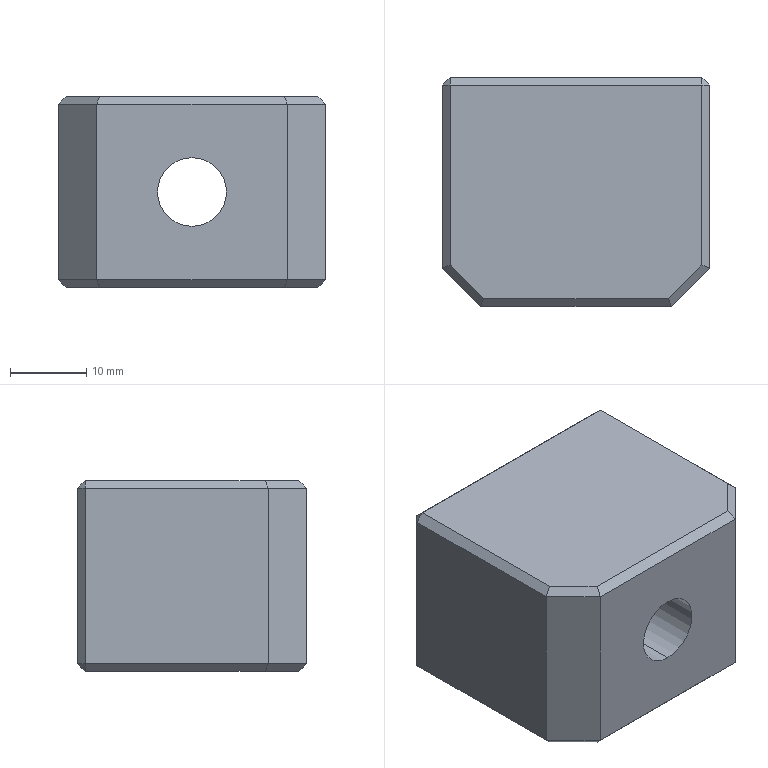Part | Creo | 1 solid | 33 faces | box 35 x 30 x 25 mm | volume 22735 mm3 | plane 27 | cylinder 4 | cone 2 | commonest cylinder face diameters 9 x2 14 x2
STEP:
#1=CARTESIAN_POINT('',(0.,0.,0.));
#2=DIRECTION('',(0.,0.,1.));
#3=DIRECTION('',(1.,0.,0.));
#4=AXIS2_PLACEMENT_3D('',#1,#2,#3);
#5=CARTESIAN_POINT('',(-59.,241.,-201.5));
#6=VERTEX_POINT('',#5);
#7=CARTESIAN_POINT('',(-59.,241.,-224.5));
#8=VERTEX_POINT('',#7);
#9=CARTESIAN_POINT('',(-59.,241.,-201.5));
#10=DIRECTION('',(0.,0.,-1.));
#11=VECTOR('',#10,23.);
#12=LINE('',#9,#11);
#13=EDGE_CURVE('',#6,#8,#12,.T.);
#14=ORIENTED_EDGE('',*,*,#13,.T.);
#15=CARTESIAN_POINT('',(-59.,217.,-224.5));
#16=VERTEX_POINT('',#15);
#17=CARTESIAN_POINT('',(-59.,241.,-224.5));
#18=DIRECTION('',(0.,-1.,0.));
#19=VECTOR('',#18,24.);
#20=LINE('',#17,#19);
#21=EDGE_CURVE('',#8,#16,#20,.T.);
#22=ORIENTED_EDGE('',*,*,#21,.T.);
#23=CARTESIAN_POINT('',(-59.,217.,-201.5));
#24=VERTEX_POINT('',#23);
#25=CARTESIAN_POINT('',(-59.,217.,-224.5));
#26=DIRECTION('',(0.,0.,1.));
#27=VECTOR('',#26,23.);
#28=LINE('',#25,#27);
#29=EDGE_CURVE('',#16,#24,#28,.T.);
#30=ORIENTED_EDGE('',*,*,#29,.T.);
#31=CARTESIAN_POINT('',(-59.,217.,-201.5));
#32=DIRECTION('',(0.,1.,0.));
#33=VECTOR('',#32,24.);
#34=LINE('',#31,#33);
#35=EDGE_CURVE('',#24,#6,#34,.T.);
#36=ORIENTED_EDGE('',*,*,#35,.T.);
#37=EDGE_LOOP('',(#14,#22,#30,#36));
#38=FACE_OUTER_BOUND('',#37,.F.);
#39=CARTESIAN_POINT('',(-59.,242.,-200.5));
#40=DIRECTION('',(-1.,0.,0.));
#41=DIRECTION('',(0.,0.,-1.));
#42=AXIS2_PLACEMENT_3D('',#39,#40,#41);
#43=PLANE('',#42);
#44=ADVANCED_FACE('',(#38),#43,.F.);
#45=CARTESIAN_POINT('',(-60.,242.,-201.5));
#46=VERTEX_POINT('',#45);
#47=CARTESIAN_POINT('',(-59.,241.,-201.5));
#48=DIRECTION('',(-0.7071,0.7071,0.));
#49=VECTOR('',#48,1.414);
#50=LINE('',#47,#49);
#51=EDGE_CURVE('',#6,#46,#50,.T.);
#52=ORIENTED_EDGE('',*,*,#51,.T.);
#53=CARTESIAN_POINT('',(-60.,242.,-224.5));
#54=VERTEX_POINT('',#53);
#55=CARTESIAN_POINT('',(-60.,242.,-224.5));
#56=DIRECTION('',(0.,0.,1.));
#57=VECTOR('',#56,23.);
#58=LINE('',#55,#57);
#59=EDGE_CURVE('',#54,#46,#58,.T.);
#60=ORIENTED_EDGE('',*,*,#59,.F.);
#61=CARTESIAN_POINT('',(-60.,242.,-224.5));
#62=DIRECTION('',(0.7071,-0.7071,0.));
#63=VECTOR('',#62,1.414);
#64=LINE('',#61,#63);
#65=EDGE_CURVE('',#54,#8,#64,.T.);
#66=ORIENTED_EDGE('',*,*,#65,.T.);
#67=ORIENTED_EDGE('',*,*,#13,.F.);
#68=EDGE_LOOP('',(#52,#60,#66,#67));
#69=FACE_OUTER_BOUND('',#68,.F.);
#70=CARTESIAN_POINT('',(-60.,242.,0.));
#71=DIRECTION('',(0.7071,0.7071,0.));
#72=DIRECTION('',(0.,0.,1.));
#73=AXIS2_PLACEMENT_3D('',#70,#71,#72);
#74=PLANE('',#73);
#75=ADVANCED_FACE('',(#69),#74,.T.);
#76=CARTESIAN_POINT('',(-60.,241.,-200.5));
#77=VERTEX_POINT('',#76);
#78=CARTESIAN_POINT('',(-60.,242.,-201.5));
#79=DIRECTION('',(0.,-0.7071,0.7071));
#80=VECTOR('',#79,1.414);
#81=LINE('',#78,#80);
#82=EDGE_CURVE('',#46,#77,#81,.T.);
#83=ORIENTED_EDGE('',*,*,#82,.F.);
#84=ORIENTED_EDGE('',*,*,#51,.F.);
#85=CARTESIAN_POINT('',(-59.,241.,-201.5));
#86=DIRECTION('',(-0.7071,0.,0.7071));
#87=VECTOR('',#86,1.414);
#88=LINE('',#85,#87);
#89=EDGE_CURVE('',#6,#77,#88,.T.);
#90=ORIENTED_EDGE('',*,*,#89,.T.);
#91=EDGE_LOOP('',(#83,#84,#90));
#92=FACE_OUTER_BOUND('',#91,.F.);
#93=CARTESIAN_POINT('',(-59.,241.,-201.5));
#94=DIRECTION('',(0.5774,0.5774,0.5774));
#95=DIRECTION('',(0.7071,0.,-0.7071));
#96=AXIS2_PLACEMENT_3D('',#93,#94,#95);
#97=PLANE('',#96);
#98=ADVANCED_FACE('',(#92),#97,.T.);
#99=CARTESIAN_POINT('',(-93.,241.,-200.5));
#100=VERTEX_POINT('',#99);
#101=CARTESIAN_POINT('',(-93.,242.,-201.5));
#102=VERTEX_POINT('',#101);
#103=CARTESIAN_POINT('',(-93.,241.,-200.5));
#104=DIRECTION('',(0.,0.7071,-0.7071));
#105=VECTOR('',#104,1.414);
#106=LINE('',#103,#105);
#107=EDGE_CURVE('',#100,#102,#106,.T.);
#108=ORIENTED_EDGE('',*,*,#107,.T.);
#109=CARTESIAN_POINT('',(-60.,242.,-201.5));
#110=DIRECTION('',(-1.,0.,0.));
#111=VECTOR('',#110,33.);
#112=LINE('',#109,#111);
#113=EDGE_CURVE('',#46,#102,#112,.T.);
#114=ORIENTED_EDGE('',*,*,#113,.F.);
#115=ORIENTED_EDGE('',*,*,#82,.T.);
#116=CARTESIAN_POINT('',(-93.,241.,-200.5));
#117=DIRECTION('',(1.,0.,0.));
#118=VECTOR('',#117,33.);
#119=LINE('',#116,#118);
#120=EDGE_CURVE('',#100,#77,#119,.T.);
#121=ORIENTED_EDGE('',*,*,#120,.F.);
#122=EDGE_LOOP('',(#108,#114,#115,#121));
#123=FACE_OUTER_BOUND('',#122,.F.);
#124=CARTESIAN_POINT('',(1.,242.,-201.5));
#125=DIRECTION('',(0.,0.7071,0.7071));
#126=DIRECTION('',(-1.,0.,0.));
#127=AXIS2_PLACEMENT_3D('',#124,#125,#126);
#128=PLANE('',#127);
#129=ADVANCED_FACE('',(#123),#128,.T.);
#130=CARTESIAN_POINT('',(-94.,241.,-201.5));
#131=VERTEX_POINT('',#130);
#132=CARTESIAN_POINT('',(-93.,241.,-200.5));
#133=DIRECTION('',(-0.7071,0.,-0.7071));
#134=VECTOR('',#133,1.414);
#135=LINE('',#132,#134);
#136=EDGE_CURVE('',#100,#131,#135,.T.);
#137=ORIENTED_EDGE('',*,*,#136,.T.);
#138=CARTESIAN_POINT('',(-93.,242.,-201.5));
#139=DIRECTION('',(-0.7071,-0.7071,0.));
#140=VECTOR('',#139,1.414);
#141=LINE('',#138,#140);
#142=EDGE_CURVE('',#102,#131,#141,.T.);
#143=ORIENTED_EDGE('',*,*,#142,.F.);
#144=ORIENTED_EDGE('',*,*,#107,.F.);
#145=EDGE_LOOP('',(#137,#143,#144));
#146=FACE_OUTER_BOUND('',#145,.F.);
#147=CARTESIAN_POINT('',(-93.,242.,-201.5));
#148=DIRECTION('',(-0.5774,0.5774,0.5774));
#149=DIRECTION('',(0.7071,0.,0.7071));
#150=AXIS2_PLACEMENT_3D('',#147,#148,#149);
#151=PLANE('',#150);
#152=ADVANCED_FACE('',(#146),#151,.T.);
#153=CARTESIAN_POINT('',(-93.,217.414,-200.5));
#154=VERTEX_POINT('',#153);
#155=CARTESIAN_POINT('',(-94.,217.,-201.5));
#156=VERTEX_POINT('',#155);
#157=CARTESIAN_POINT('',(-93.,217.414,-200.5));
#158=DIRECTION('',(-0.6786,-0.2811,-0.6786));
#159=VECTOR('',#158,1.474);
#160=LINE('',#157,#159);
#161=EDGE_CURVE('',#154,#156,#160,.T.);
#162=ORIENTED_EDGE('',*,*,#161,.T.);
#163=CARTESIAN_POINT('',(-94.,241.,-201.5));
#164=DIRECTION('',(0.,-1.,0.));
#165=VECTOR('',#164,24.);
#166=LINE('',#163,#165);
#167=EDGE_CURVE('',#131,#156,#166,.T.);
#168=ORIENTED_EDGE('',*,*,#167,.F.);
#169=ORIENTED_EDGE('',*,*,#136,.F.);
#170=CARTESIAN_POINT('',(-93.,217.414,-200.5));
#171=DIRECTION('',(0.,1.,0.));
#172=VECTOR('',#171,23.586);
#173=LINE('',#170,#172);
#174=EDGE_CURVE('',#154,#100,#173,.T.);
#175=ORIENTED_EDGE('',*,*,#174,.F.);
#176=EDGE_LOOP('',(#162,#168,#169,#175));
#177=FACE_OUTER_BOUND('',#176,.F.);
#178=CARTESIAN_POINT('',(-93.,242.,-200.5));
#179=DIRECTION('',(0.7071,0.,-0.7071));
#180=DIRECTION('',(0.,-1.,0.));
#181=AXIS2_PLACEMENT_3D('',#178,#179,#180);
#182=PLANE('',#181);
#183=ADVANCED_FACE('',(#177),#182,.F.);
#184=CARTESIAN_POINT('',(-88.586,213.,-200.5));
#185=VERTEX_POINT('',#184);
#186=CARTESIAN_POINT('',(-89.,212.,-201.5));
#187=VERTEX_POINT('',#186);
#188=CARTESIAN_POINT('',(-88.586,213.,-200.5));
#189=DIRECTION('',(-0.2811,-0.6786,-0.6786));
#190=VECTOR('',#189,1.474);
#191=LINE('',#188,#190);
#192=EDGE_CURVE('',#185,#187,#191,.T.);
#193=ORIENTED_EDGE('',*,*,#192,.T.);
#194=CARTESIAN_POINT('',(-94.,217.,-201.5));
#195=DIRECTION('',(0.7071,-0.7071,0.));
#196=VECTOR('',#195,7.071);
#197=LINE('',#194,#196);
#198=EDGE_CURVE('',#156,#187,#197,.T.);
#199=ORIENTED_EDGE('',*,*,#198,.F.);
#200=ORIENTED_EDGE('',*,*,#161,.F.);
#201=CARTESIAN_POINT('',(-93.,217.414,-200.5));
#202=DIRECTION('',(0.7071,-0.7071,0.));
#203=VECTOR('',#202,6.243);
#204=LINE('',#201,#203);
#205=EDGE_CURVE('',#154,#185,#204,.T.);
#206=ORIENTED_EDGE('',*,*,#205,.T.);
#207=EDGE_LOOP('',(#193,#199,#200,#206));
#208=FACE_OUTER_BOUND('',#207,.F.);
#209=CARTESIAN_POINT('',(-105.793,230.207,-200.5));
#210=DIRECTION('',(0.5,0.5,-0.7071));
#211=DIRECTION('',(0.7071,-0.7071,0.));
#212=AXIS2_PLACEMENT_3D('',#209,#210,#211);
#213=PLANE('',#212);
#214=ADVANCED_FACE('',(#208),#213,.F.);
#215=ORIENTED_EDGE('',*,*,#192,.F.);
#216=CARTESIAN_POINT('',(-64.414,213.,-200.5));
#217=VERTEX_POINT('',#216);
#218=CARTESIAN_POINT('',(-64.414,213.,-200.5));
#219=DIRECTION('',(-1.,0.,0.));
#220=VECTOR('',#219,24.172);
#221=LINE('',#218,#220);
#222=EDGE_CURVE('',#217,#185,#221,.T.);
#223=ORIENTED_EDGE('',*,*,#222,.F.);
#224=CARTESIAN_POINT('',(-64.,212.,-201.5));
#225=VERTEX_POINT('',#224);
#226=CARTESIAN_POINT('',(-64.,212.,-201.5));
#227=DIRECTION('',(-0.2811,0.6786,0.6786));
#228=VECTOR('',#227,1.474);
#229=LINE('',#226,#228);
#230=EDGE_CURVE('',#225,#217,#229,.T.);
#231=ORIENTED_EDGE('',*,*,#230,.F.);
#232=CARTESIAN_POINT('',(-89.,212.,-201.5));
#233=DIRECTION('',(1.,0.,0.));
#234=VECTOR('',#233,25.);
#235=LINE('',#232,#234);
#236=EDGE_CURVE('',#187,#225,#235,.T.);
#237=ORIENTED_EDGE('',*,*,#236,.F.);
#238=EDGE_LOOP('',(#215,#223,#231,#237));
#239=FACE_OUTER_BOUND('',#238,.F.);
#240=CARTESIAN_POINT('',(-94.,213.,-200.5));
#241=DIRECTION('',(0.,0.7071,-0.7071));
#242=DIRECTION('',(1.,0.,0.));
#243=AXIS2_PLACEMENT_3D('',#240,#241,#242);
#244=PLANE('',#243);
#245=ADVANCED_FACE('',(#239),#244,.F.);
#246=ORIENTED_EDGE('',*,*,#222,.T.);
#247=ORIENTED_EDGE('',*,*,#205,.F.);
#248=ORIENTED_EDGE('',*,*,#174,.T.);
#249=ORIENTED_EDGE('',*,*,#120,.T.);
#250=CARTESIAN_POINT('',(-60.,217.414,-200.5));
#251=VERTEX_POINT('',#250);
#252=CARTESIAN_POINT('',(-60.,241.,-200.5));
#253=DIRECTION('',(0.,-1.,0.));
#254=VECTOR('',#253,23.586);
#255=LINE('',#252,#254);
#256=EDGE_CURVE('',#77,#251,#255,.T.);
#257=ORIENTED_EDGE('',*,*,#256,.T.);
#258=CARTESIAN_POINT('',(-64.414,213.,-200.5));
#259=DIRECTION('',(0.7071,0.7071,0.));
#260=VECTOR('',#259,6.243);
#261=LINE('',#258,#260);
#262=EDGE_CURVE('',#217,#251,#261,.T.);
#263=ORIENTED_EDGE('',*,*,#262,.F.);
#264=EDGE_LOOP('',(#246,#247,#248,#249,#257,#263));
#265=FACE_OUTER_BOUND('',#264,.F.);
#266=CARTESIAN_POINT('',(-94.,242.,-200.5));
#267=DIRECTION('',(0.,0.,-1.));
#268=DIRECTION('',(1.,0.,0.));
#269=AXIS2_PLACEMENT_3D('',#266,#267,#268);
#270=PLANE('',#269);
#271=ADVANCED_FACE('',(#265),#270,.F.);
#272=CARTESIAN_POINT('',(-59.,217.,-201.5));
#273=DIRECTION('',(-0.6786,0.2811,0.6786));
#274=VECTOR('',#273,1.474);
#275=LINE('',#272,#274);
#276=EDGE_CURVE('',#24,#251,#275,.T.);
#277=ORIENTED_EDGE('',*,*,#276,.T.);
#278=ORIENTED_EDGE('',*,*,#256,.F.);
#279=ORIENTED_EDGE('',*,*,#89,.F.);
#280=ORIENTED_EDGE('',*,*,#35,.F.);
#281=EDGE_LOOP('',(#277,#278,#279,#280));
#282=FACE_OUTER_BOUND('',#281,.F.);
#283=CARTESIAN_POINT('',(-59.,242.,-201.5));
#284=DIRECTION('',(-0.7071,0.,-0.7071));
#285=DIRECTION('',(0.,-1.,0.));
#286=AXIS2_PLACEMENT_3D('',#283,#284,#285);
#287=PLANE('',#286);
#288=ADVANCED_FACE('',(#282),#287,.F.);
#289=ORIENTED_EDGE('',*,*,#230,.T.);
#290=ORIENTED_EDGE('',*,*,#262,.T.);
#291=ORIENTED_EDGE('',*,*,#276,.F.);
#292=CARTESIAN_POINT('',(-64.,212.,-201.5));
#293=DIRECTION('',(0.7071,0.7071,0.));
#294=VECTOR('',#293,7.071);
#295=LINE('',#292,#294);
#296=EDGE_CURVE('',#225,#24,#295,.T.);
#297=ORIENTED_EDGE('',*,*,#296,.F.);
#298=EDGE_LOOP('',(#289,#290,#291,#297));
#299=FACE_OUTER_BOUND('',#298,.F.);
#300=CARTESIAN_POINT('',(-64.707,212.707,-200.5));
#301=DIRECTION('',(-0.5,0.5,-0.7071));
#302=DIRECTION('',(0.7071,0.7071,0.));
#303=AXIS2_PLACEMENT_3D('',#300,#301,#302);
#304=PLANE('',#303);
#305=ADVANCED_FACE('',(#299),#304,.F.);
#306=CARTESIAN_POINT('',(-64.,212.,-224.5));
#307=VERTEX_POINT('',#306);
#308=CARTESIAN_POINT('',(-64.,212.,-201.5));
#309=DIRECTION('',(0.,0.,-1.));
#310=VECTOR('',#309,23.);
#311=LINE('',#308,#310);
#312=EDGE_CURVE('',#225,#307,#311,.T.);
#313=ORIENTED_EDGE('',*,*,#312,.F.);
#314=ORIENTED_EDGE('',*,*,#296,.T.);
#315=ORIENTED_EDGE('',*,*,#29,.F.);
#316=CARTESIAN_POINT('',(-59.,217.,-224.5));
#317=DIRECTION('',(-0.7071,-0.7071,0.));
#318=VECTOR('',#317,7.071);
#319=LINE('',#316,#318);
#320=EDGE_CURVE('',#16,#307,#319,.T.);
#321=ORIENTED_EDGE('',*,*,#320,.T.);
#322=EDGE_LOOP('',(#313,#314,#315,#321));
#323=FACE_OUTER_BOUND('',#322,.F.);
#324=CARTESIAN_POINT('',(-59.,217.,-200.5));
#325=DIRECTION('',(-0.7071,0.7071,0.));
#326=DIRECTION('',(0.,0.,-1.));
#327=AXIS2_PLACEMENT_3D('',#324,#325,#326);
#328=PLANE('',#327);
#329=ADVANCED_FACE('',(#323),#328,.F.);
#330=ORIENTED_EDGE('',*,*,#312,.T.);
#331=CARTESIAN_POINT('',(-89.,212.,-224.5));
#332=VERTEX_POINT('',#331);
#333=CARTESIAN_POINT('',(-64.,212.,-224.5));
#334=DIRECTION('',(-1.,0.,0.));
#335=VECTOR('',#334,25.);
#336=LINE('',#333,#335);
#337=EDGE_CURVE('',#307,#332,#336,.T.);
#338=ORIENTED_EDGE('',*,*,#337,.T.);
#339=CARTESIAN_POINT('',(-89.,212.,-224.5));
#340=DIRECTION('',(0.,0.,1.));
#341=VECTOR('',#340,23.);
#342=LINE('',#339,#341);
#343=EDGE_CURVE('',#332,#187,#342,.T.);
#344=ORIENTED_EDGE('',*,*,#343,.T.);
#345=ORIENTED_EDGE('',*,*,#236,.T.);
#346=EDGE_LOOP('',(#330,#338,#344,#345));
#347=FACE_OUTER_BOUND('',#346,.F.);
#348=CARTESIAN_POINT('',(-76.5,212.,-217.5));
#349=VERTEX_POINT('',#348);
#350=CARTESIAN_POINT('',(-76.5,212.,-208.5));
#351=VERTEX_POINT('',#350);
#352=CARTESIAN_POINT('',(-76.5,212.,-213.));
#353=DIRECTION('',(0.,1.,0.));
#354=DIRECTION('',(0.,0.,-1.));
#355=AXIS2_PLACEMENT_3D('',#352,#353,#354);
#356=CIRCLE('',#355,4.5);
#357=EDGE_CURVE('',#349,#351,#356,.T.);
#358=ORIENTED_EDGE('',*,*,#357,.F.);
#359=CARTESIAN_POINT('',(-76.5,212.,-213.));
#360=DIRECTION('',(0.,1.,0.));
#361=DIRECTION('',(0.,0.,1.));
#362=AXIS2_PLACEMENT_3D('',#359,#360,#361);
#363=CIRCLE('',#362,4.5);
#364=EDGE_CURVE('',#351,#349,#363,.T.);
#365=ORIENTED_EDGE('',*,*,#364,.F.);
#366=EDGE_LOOP('',(#358,#365));
#367=FACE_BOUND('',#366,.F.);
#368=CARTESIAN_POINT('',(1.,212.,0.));
#369=DIRECTION('',(0.,1.,0.));
#370=DIRECTION('',(0.,0.,-1.));
#371=AXIS2_PLACEMENT_3D('',#368,#369,#370);
#372=PLANE('',#371);
#373=ADVANCED_FACE('',(#347,#367),#372,.F.);
#374=CARTESIAN_POINT('',(-76.5,233.,-208.5));
#375=VERTEX_POINT('',#374);
#376=CARTESIAN_POINT('',(-76.5,233.,-217.5));
#377=VERTEX_POINT('',#376);
#378=CARTESIAN_POINT('',(-76.5,233.,-213.));
#379=DIRECTION('',(0.,-1.,0.));
#380=DIRECTION('',(0.,0.,1.));
#381=AXIS2_PLACEMENT_3D('',#378,#379,#380);
#382=CIRCLE('',#381,4.5);
#383=EDGE_CURVE('',#375,#377,#382,.T.);
#384=ORIENTED_EDGE('',*,*,#383,.T.);
#385=CARTESIAN_POINT('',(-76.5,233.,-217.5));
#386=DIRECTION('',(0.,-1.,0.));
#387=VECTOR('',#386,21.);
#388=LINE('',#385,#387);
#389=EDGE_CURVE('',#377,#349,#388,.T.);
#390=ORIENTED_EDGE('',*,*,#389,.T.);
#391=ORIENTED_EDGE('',*,*,#357,.T.);
#392=CARTESIAN_POINT('',(-76.5,233.,-208.5));
#393=DIRECTION('',(0.,-1.,0.));
#394=VECTOR('',#393,21.);
#395=LINE('',#392,#394);
#396=EDGE_CURVE('',#375,#351,#395,.T.);
#397=ORIENTED_EDGE('',*,*,#396,.F.);
#398=EDGE_LOOP('',(#384,#390,#391,#397));
#399=FACE_OUTER_BOUND('',#398,.F.);
#400=CARTESIAN_POINT('',(-76.5,42.,-213.));
#401=DIRECTION('',(0.,-1.,0.));
#402=DIRECTION('',(0.,0.,1.));
#403=AXIS2_PLACEMENT_3D('',#400,#401,#402);
#404=CYLINDRICAL_SURFACE('',#403,4.5);
#405=ADVANCED_FACE('',(#399),#404,.F.);
#406=CARTESIAN_POINT('',(-76.5,233.,-206.));
#407=VERTEX_POINT('',#406);
#408=CARTESIAN_POINT('',(-76.5,233.,-220.));
#409=VERTEX_POINT('',#408);
#410=CARTESIAN_POINT('',(-76.5,233.,-213.));
#411=DIRECTION('',(0.,1.,0.));
#412=DIRECTION('',(0.,0.,1.));
#413=AXIS2_PLACEMENT_3D('',#410,#411,#412);
#414=CIRCLE('',#413,7.);
#415=EDGE_CURVE('',#407,#409,#414,.T.);
#416=ORIENTED_EDGE('',*,*,#415,.F.);
#417=CARTESIAN_POINT('',(-76.5,233.,-213.));
#418=DIRECTION('',(0.,1.,0.));
#419=DIRECTION('',(0.,0.,-1.));
#420=AXIS2_PLACEMENT_3D('',#417,#418,#419);
#421=CIRCLE('',#420,7.);
#422=EDGE_CURVE('',#409,#407,#421,.T.);
#423=ORIENTED_EDGE('',*,*,#422,.F.);
#424=EDGE_LOOP('',(#416,#423));
#425=FACE_OUTER_BOUND('',#424,.F.);
#426=ORIENTED_EDGE('',*,*,#383,.F.);
#427=CARTESIAN_POINT('',(-76.5,233.,-213.));
#428=DIRECTION('',(0.,-1.,0.));
#429=DIRECTION('',(0.,0.,-1.));
#430=AXIS2_PLACEMENT_3D('',#427,#428,#429);
#431=CIRCLE('',#430,4.5);
#432=EDGE_CURVE('',#377,#375,#431,.T.);
#433=ORIENTED_EDGE('',*,*,#432,.F.);
#434=EDGE_LOOP('',(#426,#433));
#435=FACE_BOUND('',#434,.F.);
#436=CARTESIAN_POINT('',(-76.5,233.,-213.));
#437=DIRECTION('',(0.,-1.,0.));
#438=DIRECTION('',(0.,0.,1.));
#439=AXIS2_PLACEMENT_3D('',#436,#437,#438);
#440=PLANE('',#439);
#441=ADVANCED_FACE('',(#425,#435),#440,.F.);
#442=ORIENTED_EDGE('',*,*,#432,.T.);
#443=ORIENTED_EDGE('',*,*,#396,.T.);
#444=ORIENTED_EDGE('',*,*,#364,.T.);
#445=ORIENTED_EDGE('',*,*,#389,.F.);
#446=EDGE_LOOP('',(#442,#443,#444,#445));
#447=FACE_OUTER_BOUND('',#446,.F.);
#448=CARTESIAN_POINT('',(-76.5,42.,-213.));
#449=DIRECTION('',(0.,-1.,0.));
#450=DIRECTION('',(0.,0.,1.));
#451=AXIS2_PLACEMENT_3D('',#448,#449,#450);
#452=CYLINDRICAL_SURFACE('',#451,4.5);
#453=ADVANCED_FACE('',(#447),#452,.F.);
#454=CARTESIAN_POINT('',(-76.5,241.,-220.));
#455=VERTEX_POINT('',#454);
#456=CARTESIAN_POINT('',(-76.5,241.,-206.));
#457=VERTEX_POINT('',#456);
#458=CARTESIAN_POINT('',(-76.5,241.,-213.));
#459=DIRECTION('',(0.,-1.,0.));
#460=DIRECTION('',(0.,0.,-1.));
#461=AXIS2_PLACEMENT_3D('',#458,#459,#460);
#462=CIRCLE('',#461,7.);
#463=EDGE_CURVE('',#455,#457,#462,.T.);
#464=ORIENTED_EDGE('',*,*,#463,.T.);
#465=CARTESIAN_POINT('',(-76.5,241.,-206.));
#466=DIRECTION('',(0.,-1.,0.));
#467=VECTOR('',#466,8.);
#468=LINE('',#465,#467);
#469=EDGE_CURVE('',#457,#407,#468,.T.);
#470=ORIENTED_EDGE('',*,*,#469,.T.);
#471=ORIENTED_EDGE('',*,*,#415,.T.);
#472=CARTESIAN_POINT('',(-76.5,241.,-220.));
#473=DIRECTION('',(0.,-1.,0.));
#474=VECTOR('',#473,8.);
#475=LINE('',#472,#474);
#476=EDGE_CURVE('',#455,#409,#475,.T.);
#477=ORIENTED_EDGE('',*,*,#476,.F.);
#478=EDGE_LOOP('',(#464,#470,#471,#477));
#479=FACE_OUTER_BOUND('',#478,.F.);
#480=CARTESIAN_POINT('',(-76.5,242.,-213.));
#481=DIRECTION('',(0.,-1.,0.));
#482=DIRECTION('',(0.,0.,1.));
#483=AXIS2_PLACEMENT_3D('',#480,#481,#482);
#484=CYLINDRICAL_SURFACE('',#483,7.);
#485=ADVANCED_FACE('',(#479),#484,.F.);
#486=ORIENTED_EDGE('',*,*,#463,.F.);
#487=CARTESIAN_POINT('',(-76.5,242.,-221.));
#488=VERTEX_POINT('',#487);
#489=CARTESIAN_POINT('',(-76.5,241.,-220.));
#490=DIRECTION('',(0.,0.7071,-0.7071));
#491=VECTOR('',#490,1.414);
#492=LINE('',#489,#491);
#493=EDGE_CURVE('',#455,#488,#492,.T.);
#494=ORIENTED_EDGE('',*,*,#493,.T.);
#495=CARTESIAN_POINT('',(-76.5,242.,-205.));
#496=VERTEX_POINT('',#495);
#497=CARTESIAN_POINT('',(-76.5,242.,-213.));
#498=DIRECTION('',(0.,-1.,0.));
#499=DIRECTION('',(0.,0.,-1.));
#500=AXIS2_PLACEMENT_3D('',#497,#498,#499);
#501=CIRCLE('',#500,8.);
#502=EDGE_CURVE('',#488,#496,#501,.T.);
#503=ORIENTED_EDGE('',*,*,#502,.T.);
#504=CARTESIAN_POINT('',(-76.5,241.,-206.));
#505=DIRECTION('',(0.,0.7071,0.7071));
#506=VECTOR('',#505,1.414);
#507=LINE('',#504,#506);
#508=EDGE_CURVE('',#457,#496,#507,.T.);
#509=ORIENTED_EDGE('',*,*,#508,.F.);
#510=EDGE_LOOP('',(#486,#494,#503,#509));
#511=FACE_OUTER_BOUND('',#510,.F.);
#512=CARTESIAN_POINT('',(-76.5,241.5,-213.));
#513=DIRECTION('',(0.,1.,0.));
#514=DIRECTION('',(0.,0.,1.));
#515=AXIS2_PLACEMENT_3D('',#512,#513,#514);
#516=CONICAL_SURFACE('',#515,7.5,45.);
#517=ADVANCED_FACE('',(#511),#516,.F.);
#518=CARTESIAN_POINT('',(-76.5,241.,-213.));
#519=DIRECTION('',(0.,-1.,0.));
#520=DIRECTION('',(0.,0.,1.));
#521=AXIS2_PLACEMENT_3D('',#518,#519,#520);
#522=CIRCLE('',#521,7.);
#523=EDGE_CURVE('',#457,#455,#522,.T.);
#524=ORIENTED_EDGE('',*,*,#523,.F.);
#525=ORIENTED_EDGE('',*,*,#508,.T.);
#526=CARTESIAN_POINT('',(-76.5,242.,-213.));
#527=DIRECTION('',(0.,-1.,0.));
#528=DIRECTION('',(0.,0.,1.));
#529=AXIS2_PLACEMENT_3D('',#526,#527,#528);
#530=CIRCLE('',#529,8.);
#531=EDGE_CURVE('',#496,#488,#530,.T.);
#532=ORIENTED_EDGE('',*,*,#531,.T.);
#533=ORIENTED_EDGE('',*,*,#493,.F.);
#534=EDGE_LOOP('',(#524,#525,#532,#533));
#535=FACE_OUTER_BOUND('',#534,.F.);
#536=CARTESIAN_POINT('',(-76.5,241.5,-213.));
#537=DIRECTION('',(0.,1.,0.));
#538=DIRECTION('',(0.,0.,1.));
#539=AXIS2_PLACEMENT_3D('',#536,#537,#538);
#540=CONICAL_SURFACE('',#539,7.5,45.);
#541=ADVANCED_FACE('',(#535),#540,.F.);
#542=ORIENTED_EDGE('',*,*,#523,.T.);
#543=ORIENTED_EDGE('',*,*,#476,.T.);
#544=ORIENTED_EDGE('',*,*,#422,.T.);
#545=ORIENTED_EDGE('',*,*,#469,.F.);
#546=EDGE_LOOP('',(#542,#543,#544,#545));
#547=FACE_OUTER_BOUND('',#546,.F.);
#548=CARTESIAN_POINT('',(-76.5,242.,-213.));
#549=DIRECTION('',(0.,-1.,0.));
#550=DIRECTION('',(0.,0.,1.));
#551=AXIS2_PLACEMENT_3D('',#548,#549,#550);
#552=CYLINDRICAL_SURFACE('',#551,7.);
#553=ADVANCED_FACE('',(#547),#552,.F.);
#554=ORIENTED_EDGE('',*,*,#59,.T.);
#555=ORIENTED_EDGE('',*,*,#113,.T.);
#556=CARTESIAN_POINT('',(-93.,242.,-224.5));
#557=VERTEX_POINT('',#556);
#558=CARTESIAN_POINT('',(-93.,242.,-201.5));
#559=DIRECTION('',(0.,0.,-1.));
#560=VECTOR('',#559,23.);
#561=LINE('',#558,#560);
#562=EDGE_CURVE('',#102,#557,#561,.T.);
#563=ORIENTED_EDGE('',*,*,#562,.T.);
#564=CARTESIAN_POINT('',(-93.,242.,-224.5));
#565=DIRECTION('',(1.,0.,0.));
#566=VECTOR('',#565,33.);
#567=LINE('',#564,#566);
#568=EDGE_CURVE('',#557,#54,#567,.T.);
#569=ORIENTED_EDGE('',*,*,#568,.T.);
#570=EDGE_LOOP('',(#554,#555,#563,#569));
#571=FACE_OUTER_BOUND('',#570,.F.);
#572=ORIENTED_EDGE('',*,*,#531,.F.);
#573=ORIENTED_EDGE('',*,*,#502,.F.);
#574=EDGE_LOOP('',(#572,#573));
#575=FACE_BOUND('',#574,.F.);
#576=CARTESIAN_POINT('',(1.,242.,0.));
#577=DIRECTION('',(0.,1.,0.));
#578=DIRECTION('',(0.,0.,-1.));
#579=AXIS2_PLACEMENT_3D('',#576,#577,#578);
#580=PLANE('',#579);
#581=ADVANCED_FACE('',(#571,#575),#580,.T.);
#582=ORIENTED_EDGE('',*,*,#142,.T.);
#583=CARTESIAN_POINT('',(-94.,241.,-224.5));
#584=VERTEX_POINT('',#583);
#585=CARTESIAN_POINT('',(-94.,241.,-224.5));
#586=DIRECTION('',(0.,0.,1.));
#587=VECTOR('',#586,23.);
#588=LINE('',#585,#587);
#589=EDGE_CURVE('',#584,#131,#588,.T.);
#590=ORIENTED_EDGE('',*,*,#589,.F.);
#591=CARTESIAN_POINT('',(-94.,241.,-224.5));
#592=DIRECTION('',(0.7071,0.7071,0.));
#593=VECTOR('',#592,1.414);
#594=LINE('',#591,#593);
#595=EDGE_CURVE('',#584,#557,#594,.T.);
#596=ORIENTED_EDGE('',*,*,#595,.T.);
#597=ORIENTED_EDGE('',*,*,#562,.F.);
#598=EDGE_LOOP('',(#582,#590,#596,#597));
#599=FACE_OUTER_BOUND('',#598,.F.);
#600=CARTESIAN_POINT('',(-93.,242.,0.));
#601=DIRECTION('',(-0.7071,0.7071,0.));
#602=DIRECTION('',(0.,0.,-1.));
#603=AXIS2_PLACEMENT_3D('',#600,#601,#602);
#604=PLANE('',#603);
#605=ADVANCED_FACE('',(#599),#604,.T.);
#606=ORIENTED_EDGE('',*,*,#589,.T.);
#607=ORIENTED_EDGE('',*,*,#167,.T.);
#608=CARTESIAN_POINT('',(-94.,217.,-224.5));
#609=VERTEX_POINT('',#608);
#610=CARTESIAN_POINT('',(-94.,217.,-201.5));
#611=DIRECTION('',(0.,0.,-1.));
#612=VECTOR('',#611,23.);
#613=LINE('',#610,#612);
#614=EDGE_CURVE('',#156,#609,#613,.T.);
#615=ORIENTED_EDGE('',*,*,#614,.T.);
#616=CARTESIAN_POINT('',(-94.,217.,-224.5));
#617=DIRECTION('',(0.,1.,0.));
#618=VECTOR('',#617,24.);
#619=LINE('',#616,#618);
#620=EDGE_CURVE('',#609,#584,#619,.T.);
#621=ORIENTED_EDGE('',*,*,#620,.T.);
#622=EDGE_LOOP('',(#606,#607,#615,#621));
#623=FACE_OUTER_BOUND('',#622,.F.);
#624=CARTESIAN_POINT('',(-94.,242.,-225.5));
#625=DIRECTION('',(1.,0.,0.));
#626=DIRECTION('',(0.,0.,1.));
#627=AXIS2_PLACEMENT_3D('',#624,#625,#626);
#628=PLANE('',#627);
#629=ADVANCED_FACE('',(#623),#628,.F.);
#630=ORIENTED_EDGE('',*,*,#343,.F.);
#631=CARTESIAN_POINT('',(-89.,212.,-224.5));
#632=DIRECTION('',(-0.7071,0.7071,0.));
#633=VECTOR('',#632,7.071);
#634=LINE('',#631,#633);
#635=EDGE_CURVE('',#332,#609,#634,.T.);
#636=ORIENTED_EDGE('',*,*,#635,.T.);
#637=ORIENTED_EDGE('',*,*,#614,.F.);
#638=ORIENTED_EDGE('',*,*,#198,.T.);
#639=EDGE_LOOP('',(#630,#636,#637,#638));
#640=FACE_OUTER_BOUND('',#639,.F.);
#641=CARTESIAN_POINT('',(-94.,217.,-225.5));
#642=DIRECTION('',(0.7071,0.7071,0.));
#643=DIRECTION('',(0.,0.,1.));
#644=AXIS2_PLACEMENT_3D('',#641,#642,#643);
#645=PLANE('',#644);
#646=ADVANCED_FACE('',(#640),#645,.F.);
#647=CARTESIAN_POINT('',(-88.586,213.,-225.5));
#648=VERTEX_POINT('',#647);
#649=CARTESIAN_POINT('',(-89.,212.,-224.5));
#650=DIRECTION('',(0.2811,0.6786,-0.6786));
#651=VECTOR('',#650,1.474);
#652=LINE('',#649,#651);
#653=EDGE_CURVE('',#332,#648,#652,.T.);
#654=ORIENTED_EDGE('',*,*,#653,.T.);
#655=CARTESIAN_POINT('',(-93.,217.414,-225.5));
#656=VERTEX_POINT('',#655);
#657=CARTESIAN_POINT('',(-88.586,213.,-225.5));
#658=DIRECTION('',(-0.7071,0.7071,0.));
#659=VECTOR('',#658,6.243);
#660=LINE('',#657,#659);
#661=EDGE_CURVE('',#648,#656,#660,.T.);
#662=ORIENTED_EDGE('',*,*,#661,.T.);
#663=CARTESIAN_POINT('',(-94.,217.,-224.5));
#664=DIRECTION('',(0.6786,0.2811,-0.6786));
#665=VECTOR('',#664,1.474);
#666=LINE('',#663,#665);
#667=EDGE_CURVE('',#609,#656,#666,.T.);
#668=ORIENTED_EDGE('',*,*,#667,.F.);
#669=ORIENTED_EDGE('',*,*,#635,.F.);
#670=EDGE_LOOP('',(#654,#662,#668,#669));
#671=FACE_OUTER_BOUND('',#670,.F.);
#672=CARTESIAN_POINT('',(-88.293,212.707,-225.5));
#673=DIRECTION('',(0.5,0.5,0.7071));
#674=DIRECTION('',(-0.7071,0.7071,0.));
#675=AXIS2_PLACEMENT_3D('',#672,#673,#674);
#676=PLANE('',#675);
#677=ADVANCED_FACE('',(#671),#676,.F.);
#678=ORIENTED_EDGE('',*,*,#653,.F.);
#679=ORIENTED_EDGE('',*,*,#337,.F.);
#680=CARTESIAN_POINT('',(-64.414,213.,-225.5));
#681=VERTEX_POINT('',#680);
#682=CARTESIAN_POINT('',(-64.414,213.,-225.5));
#683=DIRECTION('',(0.2811,-0.6786,0.6786));
#684=VECTOR('',#683,1.474);
#685=LINE('',#682,#684);
#686=EDGE_CURVE('',#681,#307,#685,.T.);
#687=ORIENTED_EDGE('',*,*,#686,.F.);
#688=CARTESIAN_POINT('',(-88.586,213.,-225.5));
#689=DIRECTION('',(1.,0.,0.));
#690=VECTOR('',#689,24.172);
#691=LINE('',#688,#690);
#692=EDGE_CURVE('',#648,#681,#691,.T.);
#693=ORIENTED_EDGE('',*,*,#692,.F.);
#694=EDGE_LOOP('',(#678,#679,#687,#693));
#695=FACE_OUTER_BOUND('',#694,.F.);
#696=CARTESIAN_POINT('',(-59.,213.,-225.5));
#697=DIRECTION('',(0.,0.7071,0.7071));
#698=DIRECTION('',(-1.,0.,0.));
#699=AXIS2_PLACEMENT_3D('',#696,#697,#698);
#700=PLANE('',#699);
#701=ADVANCED_FACE('',(#695),#700,.F.);
#702=ORIENTED_EDGE('',*,*,#686,.T.);
#703=ORIENTED_EDGE('',*,*,#320,.F.);
#704=CARTESIAN_POINT('',(-60.,217.414,-225.5));
#705=VERTEX_POINT('',#704);
#706=CARTESIAN_POINT('',(-60.,217.414,-225.5));
#707=DIRECTION('',(0.6786,-0.2811,0.6786));
#708=VECTOR('',#707,1.474);
#709=LINE('',#706,#708);
#710=EDGE_CURVE('',#705,#16,#709,.T.);
#711=ORIENTED_EDGE('',*,*,#710,.F.);
#712=CARTESIAN_POINT('',(-60.,217.414,-225.5));
#713=DIRECTION('',(-0.7071,-0.7071,0.));
#714=VECTOR('',#713,6.243);
#715=LINE('',#712,#714);
#716=EDGE_CURVE('',#705,#681,#715,.T.);
#717=ORIENTED_EDGE('',*,*,#716,.T.);
#718=EDGE_LOOP('',(#702,#703,#711,#717));
#719=FACE_OUTER_BOUND('',#718,.F.);
#720=CARTESIAN_POINT('',(-47.207,230.207,-225.5));
#721=DIRECTION('',(-0.5,0.5,0.7071));
#722=DIRECTION('',(-0.7071,-0.7071,0.));
#723=AXIS2_PLACEMENT_3D('',#720,#721,#722);
#724=PLANE('',#723);
#725=ADVANCED_FACE('',(#719),#724,.F.);
#726=ORIENTED_EDGE('',*,*,#710,.T.);
#727=ORIENTED_EDGE('',*,*,#21,.F.);
#728=CARTESIAN_POINT('',(-60.,241.,-225.5));
#729=VERTEX_POINT('',#728);
#730=CARTESIAN_POINT('',(-60.,241.,-225.5));
#731=DIRECTION('',(0.7071,0.,0.7071));
#732=VECTOR('',#731,1.414);
#733=LINE('',#730,#732);
#734=EDGE_CURVE('',#729,#8,#733,.T.);
#735=ORIENTED_EDGE('',*,*,#734,.F.);
#736=CARTESIAN_POINT('',(-60.,217.414,-225.5));
#737=DIRECTION('',(0.,1.,0.));
#738=VECTOR('',#737,23.586);
#739=LINE('',#736,#738);
#740=EDGE_CURVE('',#705,#729,#739,.T.);
#741=ORIENTED_EDGE('',*,*,#740,.F.);
#742=EDGE_LOOP('',(#726,#727,#735,#741));
#743=FACE_OUTER_BOUND('',#742,.F.);
#744=CARTESIAN_POINT('',(-60.,242.,-225.5));
#745=DIRECTION('',(-0.7071,0.,0.7071));
#746=DIRECTION('',(0.,-1.,0.));
#747=AXIS2_PLACEMENT_3D('',#744,#745,#746);
#748=PLANE('',#747);
#749=ADVANCED_FACE('',(#743),#748,.F.);
#750=ORIENTED_EDGE('',*,*,#65,.F.);
#751=CARTESIAN_POINT('',(-60.,241.,-225.5));
#752=DIRECTION('',(0.,0.7071,0.7071));
#753=VECTOR('',#752,1.414);
#754=LINE('',#751,#753);
#755=EDGE_CURVE('',#729,#54,#754,.T.);
#756=ORIENTED_EDGE('',*,*,#755,.F.);
#757=ORIENTED_EDGE('',*,*,#734,.T.);
#758=EDGE_LOOP('',(#750,#756,#757));
#759=FACE_OUTER_BOUND('',#758,.F.);
#760=CARTESIAN_POINT('',(-60.,241.,-225.5));
#761=DIRECTION('',(0.5774,0.5774,-0.5774));
#762=DIRECTION('',(-0.7071,0.,-0.7071));
#763=AXIS2_PLACEMENT_3D('',#760,#761,#762);
#764=PLANE('',#763);
#765=ADVANCED_FACE('',(#759),#764,.T.);
#766=ORIENTED_EDGE('',*,*,#755,.T.);
#767=ORIENTED_EDGE('',*,*,#568,.F.);
#768=CARTESIAN_POINT('',(-93.,241.,-225.5));
#769=VERTEX_POINT('',#768);
#770=CARTESIAN_POINT('',(-93.,242.,-224.5));
#771=DIRECTION('',(0.,-0.7071,-0.7071));
#772=VECTOR('',#771,1.414);
#773=LINE('',#770,#772);
#774=EDGE_CURVE('',#557,#769,#773,.T.);
#775=ORIENTED_EDGE('',*,*,#774,.T.);
#776=CARTESIAN_POINT('',(-60.,241.,-225.5));
#777=DIRECTION('',(-1.,0.,0.));
#778=VECTOR('',#777,33.);
#779=LINE('',#776,#778);
#780=EDGE_CURVE('',#729,#769,#779,.T.);
#781=ORIENTED_EDGE('',*,*,#780,.F.);
#782=EDGE_LOOP('',(#766,#767,#775,#781));
#783=FACE_OUTER_BOUND('',#782,.F.);
#784=CARTESIAN_POINT('',(1.,242.,-224.5));
#785=DIRECTION('',(0.,0.7071,-0.7071));
#786=DIRECTION('',(1.,0.,0.));
#787=AXIS2_PLACEMENT_3D('',#784,#785,#786);
#788=PLANE('',#787);
#789=ADVANCED_FACE('',(#783),#788,.T.);
#790=CARTESIAN_POINT('',(-94.,241.,-224.5));
#791=DIRECTION('',(0.7071,0.,-0.7071));
#792=VECTOR('',#791,1.414);
#793=LINE('',#790,#792);
#794=EDGE_CURVE('',#584,#769,#793,.T.);
#795=ORIENTED_EDGE('',*,*,#794,.T.);
#796=ORIENTED_EDGE('',*,*,#774,.F.);
#797=ORIENTED_EDGE('',*,*,#595,.F.);
#798=EDGE_LOOP('',(#795,#796,#797));
#799=FACE_OUTER_BOUND('',#798,.F.);
#800=CARTESIAN_POINT('',(-93.,242.,-224.5));
#801=DIRECTION('',(-0.5774,0.5774,-0.5774));
#802=DIRECTION('',(-0.7071,0.,0.7071));
#803=AXIS2_PLACEMENT_3D('',#800,#801,#802);
#804=PLANE('',#803);
#805=ADVANCED_FACE('',(#799),#804,.T.);
#806=ORIENTED_EDGE('',*,*,#667,.T.);
#807=CARTESIAN_POINT('',(-93.,241.,-225.5));
#808=DIRECTION('',(0.,-1.,0.));
#809=VECTOR('',#808,23.586);
#810=LINE('',#807,#809);
#811=EDGE_CURVE('',#769,#656,#810,.T.);
#812=ORIENTED_EDGE('',*,*,#811,.F.);
#813=ORIENTED_EDGE('',*,*,#794,.F.);
#814=ORIENTED_EDGE('',*,*,#620,.F.);
#815=EDGE_LOOP('',(#806,#812,#813,#814));
#816=FACE_OUTER_BOUND('',#815,.F.);
#817=CARTESIAN_POINT('',(-94.,242.,-224.5));
#818=DIRECTION('',(0.7071,0.,0.7071));
#819=DIRECTION('',(0.,-1.,0.));
#820=AXIS2_PLACEMENT_3D('',#817,#818,#819);
#821=PLANE('',#820);
#822=ADVANCED_FACE('',(#816),#821,.F.);
#823=ORIENTED_EDGE('',*,*,#740,.T.);
#824=ORIENTED_EDGE('',*,*,#780,.T.);
#825=ORIENTED_EDGE('',*,*,#811,.T.);
#826=ORIENTED_EDGE('',*,*,#661,.F.);
#827=ORIENTED_EDGE('',*,*,#692,.T.);
#828=ORIENTED_EDGE('',*,*,#716,.F.);
#829=EDGE_LOOP('',(#823,#824,#825,#826,#827,#828));
#830=FACE_OUTER_BOUND('',#829,.F.);
#831=CARTESIAN_POINT('',(-59.,242.,-225.5));
#832=DIRECTION('',(0.,0.,1.));
#833=DIRECTION('',(-1.,0.,0.));
#834=AXIS2_PLACEMENT_3D('',#831,#832,#833);
#835=PLANE('',#834);
#836=ADVANCED_FACE('',(#830),#835,.F.);
#837=CLOSED_SHELL('',(#44,#75,#98,#129,#152,#183,#214,#245,#271,#288,#305,#329,#373,#405,#441,#453,#485,#517,#541,#553,#581,#605,#629,#646,#677,#701,#725,#749,#765,#789,#805,#822,#836));
#838=MANIFOLD_SOLID_BREP('',#837);
#839=(LENGTH_UNIT()NAMED_UNIT(*)SI_UNIT(.MILLI.,.METRE.));
#840=UNCERTAINTY_MEASURE_WITH_UNIT(LENGTH_MEASURE(0.005244),#839,'','');
#841=(NAMED_UNIT(*)PLANE_ANGLE_UNIT()SI_UNIT($,.RADIAN.));
#842=PLANE_ANGLE_MEASURE_WITH_UNIT(PLANE_ANGLE_MEASURE(0.01745),#841);
#843=(CONVERSION_BASED_UNIT('DEGREE',#842)NAMED_UNIT(*)PLANE_ANGLE_UNIT());
#844=(NAMED_UNIT(*)SI_UNIT($,.STERADIAN.)SOLID_ANGLE_UNIT());
#845=(GEOMETRIC_REPRESENTATION_CONTEXT(3)GLOBAL_UNCERTAINTY_ASSIGNED_CONTEXT((#840))GLOBAL_UNIT_ASSIGNED_CONTEXT((#839,#843,#844))REPRESENTATION_CONTEXT('',''));
#846=ADVANCED_BREP_SHAPE_REPRESENTATION('',(#4,#838),#845);